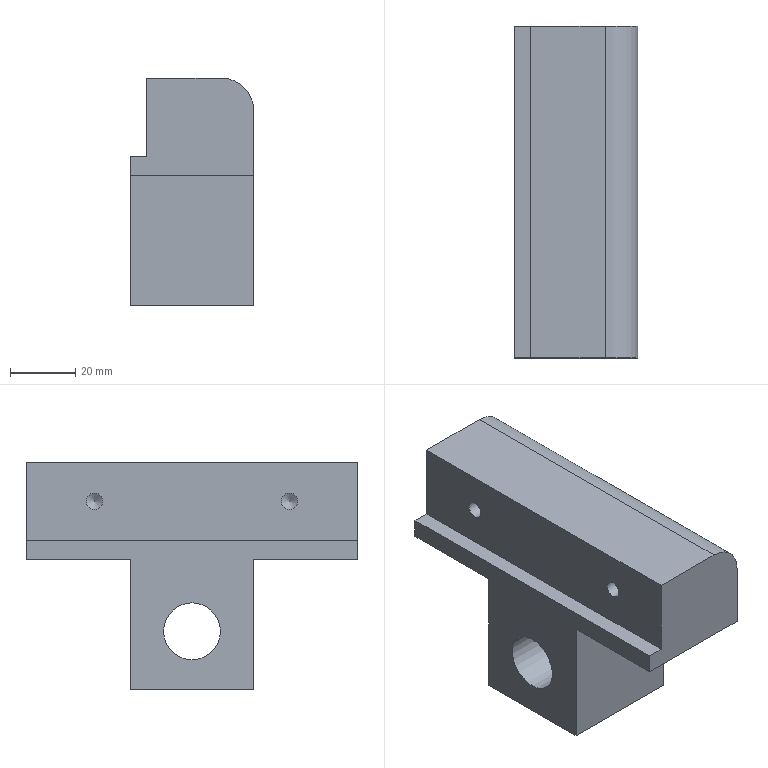Part | NX | features DATUM_CSYS 5, SIMPLE HOLE 5, SYMBOLIC_THREAD 5, SKETCH 4, HOLE PACKAGE 3, EXTRUDE 2 | 1 solid | 22 faces | box 38 x 102 x 70 mm | volume 149489 mm3 | plane 12 | cylinder 6 | cone 4 | commonest cylinder face diameters 5 x4 17.5 x1 20 x1
STEP:
#1=CARTESIAN_POINT('',(-19.,0.,9.25));
#2=VERTEX_POINT('',#1);
#3=CARTESIAN_POINT('',(-19.,0.,18.));
#4=DIRECTION('',(1.,0.,0.));
#5=DIRECTION('',(0.,0.,-1.));
#6=AXIS2_PLACEMENT_3D('',#3,#4,#5);
#7=CIRCLE('',#6,8.75);
#8=EDGE_CURVE('',#2,#2,#7,.T.);
#9=ORIENTED_EDGE('',*,*,#8,.T.);
#10=EDGE_LOOP('',(#9));
#11=FACE_BOUND('',#10,.T.);
#12=CARTESIAN_POINT('',(-19.,19.,40.));
#13=VERTEX_POINT('',#12);
#14=CARTESIAN_POINT('',(-19.,19.,0.));
#15=VERTEX_POINT('',#14);
#16=CARTESIAN_POINT('',(-19.,19.,40.));
#17=DIRECTION('',(0.,0.,-1.));
#18=VECTOR('',#17,1000.);
#19=LINE('',#16,#18);
#20=EDGE_CURVE('',#13,#15,#19,.T.);
#21=ORIENTED_EDGE('',*,*,#20,.T.);
#22=CARTESIAN_POINT('',(-19.,-19.,0.));
#23=VERTEX_POINT('',#22);
#24=CARTESIAN_POINT('',(-19.,-19.,0.));
#25=DIRECTION('',(0.,1.,0.));
#26=VECTOR('',#25,1000.);
#27=LINE('',#24,#26);
#28=EDGE_CURVE('',#23,#15,#27,.T.);
#29=ORIENTED_EDGE('',*,*,#28,.F.);
#30=CARTESIAN_POINT('',(-19.,-19.,40.));
#31=VERTEX_POINT('',#30);
#32=CARTESIAN_POINT('',(-19.,-19.,40.));
#33=DIRECTION('',(0.,0.,-1.));
#34=VECTOR('',#33,1000.);
#35=LINE('',#32,#34);
#36=EDGE_CURVE('',#31,#23,#35,.T.);
#37=ORIENTED_EDGE('',*,*,#36,.F.);
#38=CARTESIAN_POINT('',(-19.,-51.,40.));
#39=VERTEX_POINT('',#38);
#40=CARTESIAN_POINT('',(-19.,-51.,40.));
#41=DIRECTION('',(0.,1.,0.));
#42=VECTOR('',#41,1000.);
#43=LINE('',#40,#42);
#44=EDGE_CURVE('',#39,#31,#43,.T.);
#45=ORIENTED_EDGE('',*,*,#44,.F.);
#46=CARTESIAN_POINT('',(-19.,-51.,46.));
#47=VERTEX_POINT('',#46);
#48=CARTESIAN_POINT('',(-19.,-51.,46.));
#49=DIRECTION('',(0.,0.,-1.));
#50=VECTOR('',#49,1000.);
#51=LINE('',#48,#50);
#52=EDGE_CURVE('',#47,#39,#51,.T.);
#53=ORIENTED_EDGE('',*,*,#52,.F.);
#54=CARTESIAN_POINT('',(-19.,51.,46.));
#55=VERTEX_POINT('',#54);
#56=CARTESIAN_POINT('',(-19.,-51.,46.));
#57=DIRECTION('',(0.,1.,0.));
#58=VECTOR('',#57,1000.);
#59=LINE('',#56,#58);
#60=EDGE_CURVE('',#47,#55,#59,.T.);
#61=ORIENTED_EDGE('',*,*,#60,.T.);
#62=CARTESIAN_POINT('',(-19.,51.,40.));
#63=VERTEX_POINT('',#62);
#64=CARTESIAN_POINT('',(-19.,51.,46.));
#65=DIRECTION('',(0.,0.,-1.));
#66=VECTOR('',#65,1000.);
#67=LINE('',#64,#66);
#68=EDGE_CURVE('',#55,#63,#67,.T.);
#69=ORIENTED_EDGE('',*,*,#68,.T.);
#70=CARTESIAN_POINT('',(-19.,-51.,40.));
#71=DIRECTION('',(0.,1.,0.));
#72=VECTOR('',#71,1000.);
#73=LINE('',#70,#72);
#74=EDGE_CURVE('',#13,#63,#73,.T.);
#75=ORIENTED_EDGE('',*,*,#74,.F.);
#76=EDGE_LOOP('',(#21,#29,#37,#45,#53,#61,#69,#75));
#77=FACE_BOUND('',#76,.T.);
#78=CARTESIAN_POINT('',(-19.,-19.,40.));
#79=DIRECTION('',(1.,0.,0.));
#80=DIRECTION('',(0.,0.,-1.));
#81=AXIS2_PLACEMENT_3D('',#78,#79,#80);
#82=PLANE('',#81);
#83=ADVANCED_FACE('',(#11,#77),#82,.F.);
#84=CARTESIAN_POINT('',(2.5,14.,0.));
#85=VERTEX_POINT('',#84);
#86=CARTESIAN_POINT('',(0.,14.,0.));
#87=DIRECTION('',(0.,0.,1.));
#88=DIRECTION('',(1.,0.,0.));
#89=AXIS2_PLACEMENT_3D('',#86,#87,#88);
#90=CIRCLE('',#89,2.5);
#91=EDGE_CURVE('',#85,#85,#90,.T.);
#92=ORIENTED_EDGE('',*,*,#91,.T.);
#93=EDGE_LOOP('',(#92));
#94=FACE_BOUND('',#93,.T.);
#95=CARTESIAN_POINT('',(2.5,-14.,0.));
#96=VERTEX_POINT('',#95);
#97=CARTESIAN_POINT('',(0.,-14.,0.));
#98=DIRECTION('',(0.,0.,1.));
#99=DIRECTION('',(1.,0.,0.));
#100=AXIS2_PLACEMENT_3D('',#97,#98,#99);
#101=CIRCLE('',#100,2.5);
#102=EDGE_CURVE('',#96,#96,#101,.T.);
#103=ORIENTED_EDGE('',*,*,#102,.T.);
#104=EDGE_LOOP('',(#103));
#105=FACE_BOUND('',#104,.T.);
#106=CARTESIAN_POINT('',(19.,19.,0.));
#107=VERTEX_POINT('',#106);
#108=CARTESIAN_POINT('',(-19.,19.,0.));
#109=DIRECTION('',(1.,0.,0.));
#110=VECTOR('',#109,1000.);
#111=LINE('',#108,#110);
#112=EDGE_CURVE('',#15,#107,#111,.T.);
#113=ORIENTED_EDGE('',*,*,#112,.T.);
#114=CARTESIAN_POINT('',(19.,-19.,0.));
#115=VERTEX_POINT('',#114);
#116=CARTESIAN_POINT('',(19.,-19.,0.));
#117=DIRECTION('',(0.,1.,0.));
#118=VECTOR('',#117,1000.);
#119=LINE('',#116,#118);
#120=EDGE_CURVE('',#115,#107,#119,.T.);
#121=ORIENTED_EDGE('',*,*,#120,.F.);
#122=CARTESIAN_POINT('',(-19.,-19.,0.));
#123=DIRECTION('',(1.,0.,0.));
#124=VECTOR('',#123,1000.);
#125=LINE('',#122,#124);
#126=EDGE_CURVE('',#23,#115,#125,.T.);
#127=ORIENTED_EDGE('',*,*,#126,.F.);
#128=ORIENTED_EDGE('',*,*,#28,.T.);
#129=EDGE_LOOP('',(#113,#121,#127,#128));
#130=FACE_BOUND('',#129,.T.);
#131=CARTESIAN_POINT('',(-19.,-19.,0.));
#132=DIRECTION('',(0.,0.,1.));
#133=DIRECTION('',(1.,0.,0.));
#134=AXIS2_PLACEMENT_3D('',#131,#132,#133);
#135=PLANE('',#134);
#136=ADVANCED_FACE('',(#94,#105,#130),#135,.F.);
#137=CARTESIAN_POINT('',(19.,0.,26.75));
#138=VERTEX_POINT('',#137);
#139=CARTESIAN_POINT('',(19.,0.,18.));
#140=DIRECTION('',(-1.,0.,0.));
#141=DIRECTION('',(0.,0.,1.));
#142=AXIS2_PLACEMENT_3D('',#139,#140,#141);
#143=CIRCLE('',#142,8.75);
#144=EDGE_CURVE('',#138,#138,#143,.T.);
#145=ORIENTED_EDGE('',*,*,#144,.T.);
#146=EDGE_LOOP('',(#145));
#147=FACE_BOUND('',#146,.T.);
#148=CARTESIAN_POINT('',(19.,19.,40.));
#149=VERTEX_POINT('',#148);
#150=CARTESIAN_POINT('',(19.,19.,0.));
#151=DIRECTION('',(0.,0.,1.));
#152=VECTOR('',#151,1000.);
#153=LINE('',#150,#152);
#154=EDGE_CURVE('',#107,#149,#153,.T.);
#155=ORIENTED_EDGE('',*,*,#154,.T.);
#156=CARTESIAN_POINT('',(19.,51.,40.));
#157=VERTEX_POINT('',#156);
#158=CARTESIAN_POINT('',(19.,-51.,40.));
#159=DIRECTION('',(0.,1.,0.));
#160=VECTOR('',#159,1000.);
#161=LINE('',#158,#160);
#162=EDGE_CURVE('',#149,#157,#161,.T.);
#163=ORIENTED_EDGE('',*,*,#162,.T.);
#164=CARTESIAN_POINT('',(19.,51.,60.));
#165=VERTEX_POINT('',#164);
#166=CARTESIAN_POINT('',(19.,51.,40.));
#167=DIRECTION('',(0.,0.,1.));
#168=VECTOR('',#167,1000.);
#169=LINE('',#166,#168);
#170=EDGE_CURVE('',#157,#165,#169,.T.);
#171=ORIENTED_EDGE('',*,*,#170,.T.);
#172=CARTESIAN_POINT('',(19.,-51.,60.));
#173=VERTEX_POINT('',#172);
#174=CARTESIAN_POINT('',(19.,-51.,60.));
#175=DIRECTION('',(0.,1.,0.));
#176=VECTOR('',#175,1000.);
#177=LINE('',#174,#176);
#178=EDGE_CURVE('',#173,#165,#177,.T.);
#179=ORIENTED_EDGE('',*,*,#178,.F.);
#180=CARTESIAN_POINT('',(19.,-51.,40.));
#181=VERTEX_POINT('',#180);
#182=CARTESIAN_POINT('',(19.,-51.,40.));
#183=DIRECTION('',(0.,0.,1.));
#184=VECTOR('',#183,1000.);
#185=LINE('',#182,#184);
#186=EDGE_CURVE('',#181,#173,#185,.T.);
#187=ORIENTED_EDGE('',*,*,#186,.F.);
#188=CARTESIAN_POINT('',(19.,-19.,40.));
#189=VERTEX_POINT('',#188);
#190=CARTESIAN_POINT('',(19.,-51.,40.));
#191=DIRECTION('',(0.,1.,0.));
#192=VECTOR('',#191,1000.);
#193=LINE('',#190,#192);
#194=EDGE_CURVE('',#181,#189,#193,.T.);
#195=ORIENTED_EDGE('',*,*,#194,.T.);
#196=CARTESIAN_POINT('',(19.,-19.,0.));
#197=DIRECTION('',(0.,0.,1.));
#198=VECTOR('',#197,1000.);
#199=LINE('',#196,#198);
#200=EDGE_CURVE('',#115,#189,#199,.T.);
#201=ORIENTED_EDGE('',*,*,#200,.F.);
#202=ORIENTED_EDGE('',*,*,#120,.T.);
#203=EDGE_LOOP('',(#155,#163,#171,#179,#187,#195,#201,#202));
#204=FACE_BOUND('',#203,.T.);
#205=CARTESIAN_POINT('',(19.,-19.,0.));
#206=DIRECTION('',(-1.,0.,0.));
#207=DIRECTION('',(0.,0.,1.));
#208=AXIS2_PLACEMENT_3D('',#205,#206,#207);
#209=PLANE('',#208);
#210=ADVANCED_FACE('',(#147,#204),#209,.F.);
#211=CARTESIAN_POINT('',(19.,-19.,40.));
#212=DIRECTION('',(-1.,0.,0.));
#213=VECTOR('',#212,1000.);
#214=LINE('',#211,#213);
#215=EDGE_CURVE('',#189,#31,#214,.T.);
#216=ORIENTED_EDGE('',*,*,#215,.T.);
#217=ORIENTED_EDGE('',*,*,#36,.T.);
#218=ORIENTED_EDGE('',*,*,#126,.T.);
#219=ORIENTED_EDGE('',*,*,#200,.T.);
#220=EDGE_LOOP('',(#216,#217,#218,#219));
#221=FACE_BOUND('',#220,.T.);
#222=CARTESIAN_POINT('',(0.,-19.,0.));
#223=DIRECTION('',(0.,-1.,0.));
#224=DIRECTION('',(0.,0.,-1.));
#225=AXIS2_PLACEMENT_3D('',#222,#223,#224);
#226=PLANE('',#225);
#227=ADVANCED_FACE('',(#221),#226,.T.);
#228=CARTESIAN_POINT('',(19.,19.,40.));
#229=DIRECTION('',(-1.,0.,0.));
#230=VECTOR('',#229,1000.);
#231=LINE('',#228,#230);
#232=EDGE_CURVE('',#149,#13,#231,.T.);
#233=ORIENTED_EDGE('',*,*,#232,.F.);
#234=ORIENTED_EDGE('',*,*,#154,.F.);
#235=ORIENTED_EDGE('',*,*,#112,.F.);
#236=ORIENTED_EDGE('',*,*,#20,.F.);
#237=EDGE_LOOP('',(#233,#234,#235,#236));
#238=FACE_BOUND('',#237,.T.);
#239=CARTESIAN_POINT('',(0.,19.,0.));
#240=DIRECTION('',(0.,-1.,0.));
#241=DIRECTION('',(0.,0.,-1.));
#242=AXIS2_PLACEMENT_3D('',#239,#240,#241);
#243=PLANE('',#242);
#244=ADVANCED_FACE('',(#238),#243,.F.);
#245=ORIENTED_EDGE('',*,*,#162,.F.);
#246=ORIENTED_EDGE('',*,*,#232,.T.);
#247=ORIENTED_EDGE('',*,*,#74,.T.);
#248=CARTESIAN_POINT('',(-19.,51.,40.));
#249=DIRECTION('',(1.,0.,0.));
#250=VECTOR('',#249,1000.);
#251=LINE('',#248,#250);
#252=EDGE_CURVE('',#63,#157,#251,.T.);
#253=ORIENTED_EDGE('',*,*,#252,.T.);
#254=EDGE_LOOP('',(#245,#246,#247,#253));
#255=FACE_BOUND('',#254,.T.);
#256=CARTESIAN_POINT('',(-19.,-51.,40.));
#257=DIRECTION('',(0.,0.,1.));
#258=DIRECTION('',(1.,0.,0.));
#259=AXIS2_PLACEMENT_3D('',#256,#257,#258);
#260=PLANE('',#259);
#261=ADVANCED_FACE('',(#255),#260,.F.);
#262=CARTESIAN_POINT('',(9.,51.,70.));
#263=VERTEX_POINT('',#262);
#264=CARTESIAN_POINT('',(9.,51.,60.));
#265=DIRECTION('',(0.,-1.,0.));
#266=DIRECTION('',(1.,0.,0.));
#267=AXIS2_PLACEMENT_3D('',#264,#265,#266);
#268=CIRCLE('',#267,10.);
#269=EDGE_CURVE('',#165,#263,#268,.T.);
#270=ORIENTED_EDGE('',*,*,#269,.T.);
#271=CARTESIAN_POINT('',(9.,-51.,70.));
#272=VERTEX_POINT('',#271);
#273=CARTESIAN_POINT('',(9.,-51.,70.));
#274=DIRECTION('',(0.,1.,0.));
#275=VECTOR('',#274,1000.);
#276=LINE('',#273,#275);
#277=EDGE_CURVE('',#272,#263,#276,.T.);
#278=ORIENTED_EDGE('',*,*,#277,.F.);
#279=CARTESIAN_POINT('',(9.,-51.,60.));
#280=DIRECTION('',(0.,-1.,0.));
#281=DIRECTION('',(1.,0.,0.));
#282=AXIS2_PLACEMENT_3D('',#279,#280,#281);
#283=CIRCLE('',#282,10.);
#284=EDGE_CURVE('',#173,#272,#283,.T.);
#285=ORIENTED_EDGE('',*,*,#284,.F.);
#286=ORIENTED_EDGE('',*,*,#178,.T.);
#287=EDGE_LOOP('',(#270,#278,#285,#286));
#288=FACE_BOUND('',#287,.T.);
#289=CARTESIAN_POINT('',(9.,-51.,60.));
#290=DIRECTION('',(0.,1.,0.));
#291=DIRECTION('',(0.,0.,1.));
#292=AXIS2_PLACEMENT_3D('',#289,#290,#291);
#293=CYLINDRICAL_SURFACE('',#292,10.);
#294=ADVANCED_FACE('',(#288),#293,.T.);
#295=CARTESIAN_POINT('',(-14.,51.,70.));
#296=VERTEX_POINT('',#295);
#297=CARTESIAN_POINT('',(9.,51.,70.));
#298=DIRECTION('',(-1.,0.,0.));
#299=VECTOR('',#298,1000.);
#300=LINE('',#297,#299);
#301=EDGE_CURVE('',#263,#296,#300,.T.);
#302=ORIENTED_EDGE('',*,*,#301,.T.);
#303=CARTESIAN_POINT('',(-14.,-51.,70.));
#304=VERTEX_POINT('',#303);
#305=CARTESIAN_POINT('',(-14.,-51.,70.));
#306=DIRECTION('',(0.,1.,0.));
#307=VECTOR('',#306,1000.);
#308=LINE('',#305,#307);
#309=EDGE_CURVE('',#304,#296,#308,.T.);
#310=ORIENTED_EDGE('',*,*,#309,.F.);
#311=CARTESIAN_POINT('',(9.,-51.,70.));
#312=DIRECTION('',(-1.,0.,0.));
#313=VECTOR('',#312,1000.);
#314=LINE('',#311,#313);
#315=EDGE_CURVE('',#272,#304,#314,.T.);
#316=ORIENTED_EDGE('',*,*,#315,.F.);
#317=ORIENTED_EDGE('',*,*,#277,.T.);
#318=EDGE_LOOP('',(#302,#310,#316,#317));
#319=FACE_BOUND('',#318,.T.);
#320=CARTESIAN_POINT('',(9.,-51.,70.));
#321=DIRECTION('',(0.,0.,-1.));
#322=DIRECTION('',(-1.,0.,0.));
#323=AXIS2_PLACEMENT_3D('',#320,#321,#322);
#324=PLANE('',#323);
#325=ADVANCED_FACE('',(#319),#324,.F.);
#326=CARTESIAN_POINT('',(-14.,30.,55.5));
#327=VERTEX_POINT('',#326);
#328=CARTESIAN_POINT('',(-14.,30.,58.));
#329=DIRECTION('',(1.,0.,0.));
#330=DIRECTION('',(0.,0.,-1.));
#331=AXIS2_PLACEMENT_3D('',#328,#329,#330);
#332=CIRCLE('',#331,2.5);
#333=EDGE_CURVE('',#327,#327,#332,.T.);
#334=ORIENTED_EDGE('',*,*,#333,.T.);
#335=EDGE_LOOP('',(#334));
#336=FACE_BOUND('',#335,.T.);
#337=CARTESIAN_POINT('',(-14.,-30.,55.5));
#338=VERTEX_POINT('',#337);
#339=CARTESIAN_POINT('',(-14.,-30.,58.));
#340=DIRECTION('',(1.,0.,0.));
#341=DIRECTION('',(0.,0.,-1.));
#342=AXIS2_PLACEMENT_3D('',#339,#340,#341);
#343=CIRCLE('',#342,2.5);
#344=EDGE_CURVE('',#338,#338,#343,.T.);
#345=ORIENTED_EDGE('',*,*,#344,.T.);
#346=EDGE_LOOP('',(#345));
#347=FACE_BOUND('',#346,.T.);
#348=CARTESIAN_POINT('',(-14.,51.,46.));
#349=VERTEX_POINT('',#348);
#350=CARTESIAN_POINT('',(-14.,51.,70.));
#351=DIRECTION('',(0.,0.,-1.));
#352=VECTOR('',#351,1000.);
#353=LINE('',#350,#352);
#354=EDGE_CURVE('',#296,#349,#353,.T.);
#355=ORIENTED_EDGE('',*,*,#354,.T.);
#356=CARTESIAN_POINT('',(-14.,-51.,46.));
#357=VERTEX_POINT('',#356);
#358=CARTESIAN_POINT('',(-14.,-51.,46.));
#359=DIRECTION('',(0.,1.,0.));
#360=VECTOR('',#359,1000.);
#361=LINE('',#358,#360);
#362=EDGE_CURVE('',#357,#349,#361,.T.);
#363=ORIENTED_EDGE('',*,*,#362,.F.);
#364=CARTESIAN_POINT('',(-14.,-51.,70.));
#365=DIRECTION('',(0.,0.,-1.));
#366=VECTOR('',#365,1000.);
#367=LINE('',#364,#366);
#368=EDGE_CURVE('',#304,#357,#367,.T.);
#369=ORIENTED_EDGE('',*,*,#368,.F.);
#370=ORIENTED_EDGE('',*,*,#309,.T.);
#371=EDGE_LOOP('',(#355,#363,#369,#370));
#372=FACE_BOUND('',#371,.T.);
#373=CARTESIAN_POINT('',(-14.,-51.,70.));
#374=DIRECTION('',(1.,0.,0.));
#375=DIRECTION('',(0.,0.,-1.));
#376=AXIS2_PLACEMENT_3D('',#373,#374,#375);
#377=PLANE('',#376);
#378=ADVANCED_FACE('',(#336,#347,#372),#377,.F.);
#379=CARTESIAN_POINT('',(-14.,51.,46.));
#380=DIRECTION('',(-1.,0.,0.));
#381=VECTOR('',#380,1000.);
#382=LINE('',#379,#381);
#383=EDGE_CURVE('',#349,#55,#382,.T.);
#384=ORIENTED_EDGE('',*,*,#383,.T.);
#385=ORIENTED_EDGE('',*,*,#60,.F.);
#386=CARTESIAN_POINT('',(-14.,-51.,46.));
#387=DIRECTION('',(-1.,0.,0.));
#388=VECTOR('',#387,1000.);
#389=LINE('',#386,#388);
#390=EDGE_CURVE('',#357,#47,#389,.T.);
#391=ORIENTED_EDGE('',*,*,#390,.F.);
#392=ORIENTED_EDGE('',*,*,#362,.T.);
#393=EDGE_LOOP('',(#384,#385,#391,#392));
#394=FACE_BOUND('',#393,.T.);
#395=CARTESIAN_POINT('',(-14.,-51.,46.));
#396=DIRECTION('',(0.,0.,-1.));
#397=DIRECTION('',(-1.,0.,0.));
#398=AXIS2_PLACEMENT_3D('',#395,#396,#397);
#399=PLANE('',#398);
#400=ADVANCED_FACE('',(#394),#399,.F.);
#401=ORIENTED_EDGE('',*,*,#215,.F.);
#402=ORIENTED_EDGE('',*,*,#194,.F.);
#403=CARTESIAN_POINT('',(-19.,-51.,40.));
#404=DIRECTION('',(1.,0.,0.));
#405=VECTOR('',#404,1000.);
#406=LINE('',#403,#405);
#407=EDGE_CURVE('',#39,#181,#406,.T.);
#408=ORIENTED_EDGE('',*,*,#407,.F.);
#409=ORIENTED_EDGE('',*,*,#44,.T.);
#410=EDGE_LOOP('',(#401,#402,#408,#409));
#411=FACE_BOUND('',#410,.T.);
#412=CARTESIAN_POINT('',(-19.,-51.,40.));
#413=DIRECTION('',(0.,0.,1.));
#414=DIRECTION('',(1.,0.,0.));
#415=AXIS2_PLACEMENT_3D('',#412,#413,#414);
#416=PLANE('',#415);
#417=ADVANCED_FACE('',(#411),#416,.F.);
#418=ORIENTED_EDGE('',*,*,#284,.T.);
#419=ORIENTED_EDGE('',*,*,#315,.T.);
#420=ORIENTED_EDGE('',*,*,#368,.T.);
#421=ORIENTED_EDGE('',*,*,#390,.T.);
#422=ORIENTED_EDGE('',*,*,#52,.T.);
#423=ORIENTED_EDGE('',*,*,#407,.T.);
#424=ORIENTED_EDGE('',*,*,#186,.T.);
#425=EDGE_LOOP('',(#418,#419,#420,#421,#422,#423,#424));
#426=FACE_BOUND('',#425,.T.);
#427=CARTESIAN_POINT('',(9.,-51.,60.));
#428=DIRECTION('',(0.,-1.,0.));
#429=DIRECTION('',(0.,0.,-1.));
#430=AXIS2_PLACEMENT_3D('',#427,#428,#429);
#431=PLANE('',#430);
#432=ADVANCED_FACE('',(#426),#431,.T.);
#433=ORIENTED_EDGE('',*,*,#269,.F.);
#434=ORIENTED_EDGE('',*,*,#170,.F.);
#435=ORIENTED_EDGE('',*,*,#252,.F.);
#436=ORIENTED_EDGE('',*,*,#68,.F.);
#437=ORIENTED_EDGE('',*,*,#383,.F.);
#438=ORIENTED_EDGE('',*,*,#354,.F.);
#439=ORIENTED_EDGE('',*,*,#301,.F.);
#440=EDGE_LOOP('',(#433,#434,#435,#436,#437,#438,#439));
#441=FACE_BOUND('',#440,.T.);
#442=CARTESIAN_POINT('',(9.,51.,60.));
#443=DIRECTION('',(0.,-1.,0.));
#444=DIRECTION('',(0.,0.,-1.));
#445=AXIS2_PLACEMENT_3D('',#442,#443,#444);
#446=PLANE('',#445);
#447=ADVANCED_FACE('',(#441),#446,.F.);
#448=ORIENTED_EDGE('',*,*,#8,.F.);
#449=EDGE_LOOP('',(#448));
#450=FACE_BOUND('',#449,.T.);
#451=ORIENTED_EDGE('',*,*,#144,.F.);
#452=EDGE_LOOP('',(#451));
#453=FACE_BOUND('',#452,.T.);
#454=CARTESIAN_POINT('',(-19.,0.,18.));
#455=DIRECTION('',(1.,0.,0.));
#456=DIRECTION('',(0.,0.,-1.));
#457=AXIS2_PLACEMENT_3D('',#454,#455,#456);
#458=CYLINDRICAL_SURFACE('',#457,8.75);
#459=ADVANCED_FACE('',(#450,#453),#458,.F.);
#460=CARTESIAN_POINT('',(2.5,-14.,12.));
#461=VERTEX_POINT('',#460);
#462=CARTESIAN_POINT('',(0.,-14.,12.));
#463=DIRECTION('',(0.,0.,1.));
#464=DIRECTION('',(1.,0.,0.));
#465=AXIS2_PLACEMENT_3D('',#462,#463,#464);
#466=CIRCLE('',#465,2.5);
#467=EDGE_CURVE('',#461,#461,#466,.F.);
#468=ORIENTED_EDGE('',*,*,#467,.T.);
#469=EDGE_LOOP('',(#468));
#470=FACE_BOUND('',#469,.T.);
#471=CARTESIAN_POINT('',(0.,-14.,13.502));
#472=VERTEX_POINT('',#471);
#473=VERTEX_LOOP('',#472);
#474=FACE_BOUND('',#473,.T.);
#475=CARTESIAN_POINT('',(0.,-14.,12.));
#476=DIRECTION('',(0.,0.,-1.));
#477=DIRECTION('',(-1.,0.,0.));
#478=AXIS2_PLACEMENT_3D('',#475,#476,#477);
#479=CONICAL_SURFACE('',#478,2.5,1.03);
#480=ADVANCED_FACE('',(#470,#474),#479,.F.);
#481=ORIENTED_EDGE('',*,*,#467,.F.);
#482=EDGE_LOOP('',(#481));
#483=FACE_BOUND('',#482,.T.);
#484=ORIENTED_EDGE('',*,*,#102,.F.);
#485=EDGE_LOOP('',(#484));
#486=FACE_BOUND('',#485,.T.);
#487=CARTESIAN_POINT('',(0.,-14.,0.));
#488=DIRECTION('',(0.,0.,1.));
#489=DIRECTION('',(1.,0.,0.));
#490=AXIS2_PLACEMENT_3D('',#487,#488,#489);
#491=CYLINDRICAL_SURFACE('',#490,2.5);
#492=ADVANCED_FACE('',(#483,#486),#491,.F.);
#493=CARTESIAN_POINT('',(2.5,14.,12.));
#494=VERTEX_POINT('',#493);
#495=CARTESIAN_POINT('',(0.,14.,12.));
#496=DIRECTION('',(0.,0.,1.));
#497=DIRECTION('',(1.,0.,0.));
#498=AXIS2_PLACEMENT_3D('',#495,#496,#497);
#499=CIRCLE('',#498,2.5);
#500=EDGE_CURVE('',#494,#494,#499,.F.);
#501=ORIENTED_EDGE('',*,*,#500,.T.);
#502=EDGE_LOOP('',(#501));
#503=FACE_BOUND('',#502,.T.);
#504=CARTESIAN_POINT('',(0.,14.,13.502));
#505=VERTEX_POINT('',#504);
#506=VERTEX_LOOP('',#505);
#507=FACE_BOUND('',#506,.T.);
#508=CARTESIAN_POINT('',(0.,14.,12.));
#509=DIRECTION('',(0.,0.,-1.));
#510=DIRECTION('',(-1.,0.,0.));
#511=AXIS2_PLACEMENT_3D('',#508,#509,#510);
#512=CONICAL_SURFACE('',#511,2.5,1.03);
#513=ADVANCED_FACE('',(#503,#507),#512,.F.);
#514=ORIENTED_EDGE('',*,*,#500,.F.);
#515=EDGE_LOOP('',(#514));
#516=FACE_BOUND('',#515,.T.);
#517=ORIENTED_EDGE('',*,*,#91,.F.);
#518=EDGE_LOOP('',(#517));
#519=FACE_BOUND('',#518,.T.);
#520=CARTESIAN_POINT('',(0.,14.,0.));
#521=DIRECTION('',(0.,0.,1.));
#522=DIRECTION('',(1.,0.,0.));
#523=AXIS2_PLACEMENT_3D('',#520,#521,#522);
#524=CYLINDRICAL_SURFACE('',#523,2.5);
#525=ADVANCED_FACE('',(#516,#519),#524,.F.);
#526=CARTESIAN_POINT('',(-2.,-30.,55.5));
#527=VERTEX_POINT('',#526);
#528=CARTESIAN_POINT('',(-2.,-30.,58.));
#529=DIRECTION('',(1.,0.,0.));
#530=DIRECTION('',(0.,0.,-1.));
#531=AXIS2_PLACEMENT_3D('',#528,#529,#530);
#532=CIRCLE('',#531,2.5);
#533=EDGE_CURVE('',#527,#527,#532,.F.);
#534=ORIENTED_EDGE('',*,*,#533,.T.);
#535=EDGE_LOOP('',(#534));
#536=FACE_BOUND('',#535,.T.);
#537=CARTESIAN_POINT('',(-0.4978,-30.,58.));
#538=VERTEX_POINT('',#537);
#539=VERTEX_LOOP('',#538);
#540=FACE_BOUND('',#539,.T.);
#541=CARTESIAN_POINT('',(-2.,-30.,58.));
#542=DIRECTION('',(-1.,0.,0.));
#543=DIRECTION('',(0.,0.,1.));
#544=AXIS2_PLACEMENT_3D('',#541,#542,#543);
#545=CONICAL_SURFACE('',#544,2.5,1.03);
#546=ADVANCED_FACE('',(#536,#540),#545,.F.);
#547=ORIENTED_EDGE('',*,*,#533,.F.);
#548=EDGE_LOOP('',(#547));
#549=FACE_BOUND('',#548,.T.);
#550=ORIENTED_EDGE('',*,*,#344,.F.);
#551=EDGE_LOOP('',(#550));
#552=FACE_BOUND('',#551,.T.);
#553=CARTESIAN_POINT('',(-14.,-30.,58.));
#554=DIRECTION('',(1.,0.,0.));
#555=DIRECTION('',(0.,0.,-1.));
#556=AXIS2_PLACEMENT_3D('',#553,#554,#555);
#557=CYLINDRICAL_SURFACE('',#556,2.5);
#558=ADVANCED_FACE('',(#549,#552),#557,.F.);
#559=CARTESIAN_POINT('',(-2.,30.,55.5));
#560=VERTEX_POINT('',#559);
#561=CARTESIAN_POINT('',(-2.,30.,58.));
#562=DIRECTION('',(1.,0.,0.));
#563=DIRECTION('',(0.,0.,-1.));
#564=AXIS2_PLACEMENT_3D('',#561,#562,#563);
#565=CIRCLE('',#564,2.5);
#566=EDGE_CURVE('',#560,#560,#565,.F.);
#567=ORIENTED_EDGE('',*,*,#566,.T.);
#568=EDGE_LOOP('',(#567));
#569=FACE_BOUND('',#568,.T.);
#570=CARTESIAN_POINT('',(-0.4978,30.,58.));
#571=VERTEX_POINT('',#570);
#572=VERTEX_LOOP('',#571);
#573=FACE_BOUND('',#572,.T.);
#574=CARTESIAN_POINT('',(-2.,30.,58.));
#575=DIRECTION('',(-1.,0.,0.));
#576=DIRECTION('',(0.,0.,1.));
#577=AXIS2_PLACEMENT_3D('',#574,#575,#576);
#578=CONICAL_SURFACE('',#577,2.5,1.03);
#579=ADVANCED_FACE('',(#569,#573),#578,.F.);
#580=ORIENTED_EDGE('',*,*,#566,.F.);
#581=EDGE_LOOP('',(#580));
#582=FACE_BOUND('',#581,.T.);
#583=ORIENTED_EDGE('',*,*,#333,.F.);
#584=EDGE_LOOP('',(#583));
#585=FACE_BOUND('',#584,.T.);
#586=CARTESIAN_POINT('',(-14.,30.,58.));
#587=DIRECTION('',(1.,0.,0.));
#588=DIRECTION('',(0.,0.,-1.));
#589=AXIS2_PLACEMENT_3D('',#586,#587,#588);
#590=CYLINDRICAL_SURFACE('',#589,2.5);
#591=ADVANCED_FACE('',(#582,#585),#590,.F.);
#592=CLOSED_SHELL('',(#83,#136,#210,#227,#244,#261,#294,#325,#378,#400,#417,#432,#447,#459,#480,#492,#513,#525,#546,#558,#579,#591));
#593=MANIFOLD_SOLID_BREP('',#592);
#594=(LENGTH_UNIT()NAMED_UNIT(*)SI_UNIT(.MILLI.,.METRE.));
#595=UNCERTAINTY_MEASURE_WITH_UNIT(LENGTH_MEASURE(0.00001),#594,'','');
#596=(NAMED_UNIT(*)PLANE_ANGLE_UNIT()SI_UNIT($,.RADIAN.));
#597=(NAMED_UNIT(*)SI_UNIT($,.STERADIAN.)SOLID_ANGLE_UNIT());
#598=(GEOMETRIC_REPRESENTATION_CONTEXT(3)GLOBAL_UNCERTAINTY_ASSIGNED_CONTEXT((#595))GLOBAL_UNIT_ASSIGNED_CONTEXT((#594,#596,#597))REPRESENTATION_CONTEXT('',''));
#599=ADVANCED_BREP_SHAPE_REPRESENTATION('',(#593),#598);